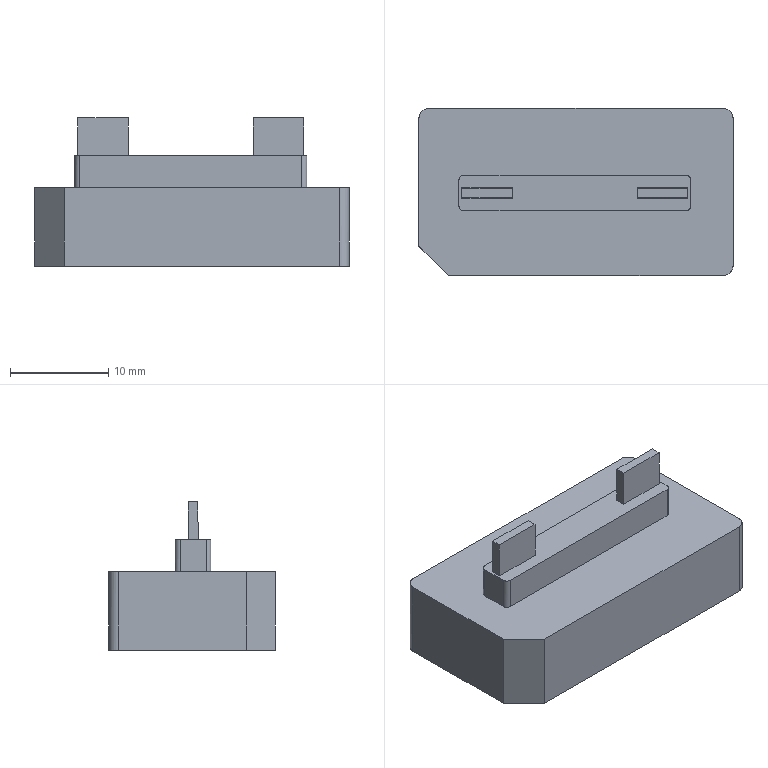NC program | PowerMill | posted by the shop | part box 32 x 17 x 15.109 mm
Lines 3099 to 3803 of 35413:
( TOOL ID   D10_1_1 )
( TOOL DIA. 10. TIP RAD 0 LENGTH 70.28 )
( Z = -4.199 )
T3 M6
T10
G91 G28 Z0
G0 G90 G54
M08
S8500 M3
X0 Y0 M8
G43 Z11.799 H3
X11.793 Y12.269
Z-2.999
G1 Z-4.199 F360
X11.412 Y7.008 F600
X8.803 Y5.703
X11.383
X11.779 Y5.688
X12.173 Y5.644
X12.562 Y5.57
X12.945 Y5.467
G2 X13.682 Y5.178 I-1.935 J-6.015
G1 X14.033 Y4.993
X14.368 Y4.782
X14.687 Y4.547
X14.988 Y4.288
X15.268 Y4.008
X15.526 Y3.707
X15.762 Y3.389
X15.973 Y3.053
X16.158 Y2.702
X16.316 Y2.339
X16.447 Y1.965
X16.55 Y1.582
X16.623 Y1.193
X16.668 Y.799
X16.683 Y.403
Y-.627
X16.668 Y-1.023
X16.623 Y-1.417
X16.55 Y-1.806
X16.447 Y-2.189
X16.316 Y-2.563
X16.158 Y-2.927
X15.973 Y-3.277
X15.762 Y-3.613
X15.526 Y-3.932
X15.268 Y-4.232
X14.988 Y-4.512
X14.687 Y-4.771
G2 X14.033 Y-5.217 I-3.905 J5.025
G1 X13.682 Y-5.402
X13.319 Y-5.561
X12.945 Y-5.692
X12.562 Y-5.794
X12.173 Y-5.868
X11.779 Y-5.912
X11.383 Y-5.927
X6.223
X5.827 Y-5.912
X5.433 Y-5.868
X5.044 Y-5.794
X4.661 Y-5.692
X4.287 Y-5.561
X3.923 Y-5.402
X3.573 Y-5.217
X3.237 Y-5.006
X2.919 Y-4.771
G2 X2.338 Y-4.232 I3.952 J4.841
G1 X2.079 Y-3.932
G2 X1.633 Y-3.277 I4.757 J3.723
G1 X1.448 Y-2.927
X1.289 Y-2.563
X1.158 Y-2.189
X1.056 Y-1.806
X.982 Y-1.417
X.938 Y-1.023
X.923 Y-.627
Y.403
X.938 Y.799
G2 X1.056 Y1.582 I6.328 J-.553
G1 X1.158 Y1.965
X1.289 Y2.339
X1.448 Y2.702
X1.633 Y3.053
X1.844 Y3.389
X2.079 Y3.707
X2.338 Y4.008
G2 X2.919 Y4.547 I4.57 J-4.343
G1 X3.237 Y4.782
X3.573 Y4.993
X3.923 Y5.178
X4.287 Y5.337
X4.661 Y5.467
X5.044 Y5.57
X5.433 Y5.644
X5.827 Y5.688
X6.223 Y5.703
X8.803
X8.869 Y5.716 Z-4.196
X8.94 Y5.768 Z-4.186
X8.978 Y5.864 Z-4.167
X8.953 Y5.964 Z-4.147
X8.889 Y6.025 Z-4.135
X8.825 Y6.046 Z-4.13
X6.619 Y6.315 Z-4.077
X6.196 Y6.335 Z-4.068
X5.767 Y6.29 Z-4.063
X5.348 Y6.18 Z-4.061
X4.952 Y6.008 Z-4.063
X4.594 Y5.783 Z-4.069
X3.226 Y4.773 Z-4.099
X3.095 Y4.677 Z-4.102 F360
X2.919 Y4.547 Z-4.105
X2.62 Y4.286 Z-4.112
X2.338 Y4.008 Z-4.119
X2.079 Y3.707 Z-4.126
X1.931 Y3.507 Z-4.131
X1.844 Y3.389 Z-4.133
X1.633 Y3.053 Z-4.14
X1.5 Y2.801 Z-4.145
X1.448 Y2.702 Z-4.147
X1.289 Y2.339 Z-4.154
X1.158 Y1.965 Z-4.161
X1.056 Y1.582 Z-4.168
X.985 Y1.192 Z-4.175
X.938 Y.799 Z-4.182
X.935 Y.73 Z-4.183
X.923 Y.403 Z-4.188
Y-.189 Z-4.199
X-1.451 Y2.115 F600
X-1.398 Y1.965
X-1.296 Y1.582
X-1.222 Y1.193
X-1.178 Y.799
X-1.163 Y.403
X-1.169 Y-.774
X-1.178 Y-1.023
X-1.222 Y-1.417
X-1.296 Y-1.806
X-1.398 Y-2.189
X-1.529 Y-2.563
X-1.688 Y-2.927
X-1.873 Y-3.277
X-2.084 Y-3.613
X-2.319 Y-3.932
X-2.578 Y-4.232
X-2.858 Y-4.512
X-3.159 Y-4.771
X-3.477 Y-5.006
X-3.813 Y-5.217
X-4.163 Y-5.402
G2 X-4.901 Y-5.692 I-2.699 J5.793
G1 X-5.284 Y-5.794
X-5.673 Y-5.868
X-6.067 Y-5.912
X-6.463 Y-5.927
X-11.623
X-12.019 Y-5.912
X-12.413 Y-5.868
G2 X-13.185 Y-5.692 I.989 J6.112
G1 X-13.559 Y-5.561
X-13.922 Y-5.402
X-14.273 Y-5.217
X-14.608 Y-5.006
X-14.927 Y-4.771
X-15.12 Y-4.606
X-15.508 Y-4.232
X-15.766 Y-3.932
G2 X-16.213 Y-3.277 I4.862 J3.795
G1 X-16.398 Y-2.927
G2 X-16.687 Y-2.189 I5.522 J2.593
G1 X-16.79 Y-1.806
X-16.863 Y-1.417
X-16.908 Y-1.023
X-16.923 Y-.627
Y.403
X-16.908 Y.799
G2 X-16.79 Y1.582 I6.194 J-.533
G1 X-16.687 Y1.965
X-16.556 Y2.339
X-16.398 Y2.703
X-16.213 Y3.053
X-16.002 Y3.389
X-15.766 Y3.707
X-15.508 Y4.008
X-15.228 Y4.288
X-14.927 Y4.547
X-14.608 Y4.782
X-14.273 Y4.993
X-13.922 Y5.178
X-13.559 Y5.337
X-13.185 Y5.467
G2 X-12.413 Y5.644 I1.802 J-6.114
G1 X-12.019 Y5.688
X-11.623 Y5.703
X-6.463
X-6.067 Y5.688
X-5.673 Y5.644
X-5.284 Y5.57
X-4.901 Y5.467
X-4.527 Y5.337
X-4.163 Y5.178
X-3.813 Y4.993
X-3.402 Y4.726
X-3.159 Y4.547
X-2.858 Y4.288
G2 X-2.319 Y3.707 I-4.255 J-4.488
G1 X-2.084 Y3.389
G2 X-1.688 Y2.702 I-5.017 J-3.354
G1 X-1.529 Y2.339
X-1.451 Y2.115
G0 Z3.999
G1 X-10.478 Y-11.178 F10000
G0 Z.849
G1 Z-.351 F360
X-10.479 Y-5.903 F600
X-10.6 Y-1.478
X-8.043 Y-1.408
G3 X-6.882 Y-.156 I-.033 J1.195
G1 X-6.892 Y.055
G3 X-8.516 Y1.112 I-1.194 J-.058
G1 X-10.932 Y.179
G3 X-10.6 Y-1.478 I.309 J-.8
G1 X-10.479 Y-5.903
G0 Z3.999
G1 X7.132 Y-11.178 F10000
G0 Z.849
G1 Z-.351 F360
X7.131 Y-5.903 F600
X7.179 Y-1.356
X9.862 Y-1.384
G3 X11.064 Y-.126 I.012 J1.192
G1 X11.055 Y.031
G3 X9.459 Y1.085 I-1.19 J-.066
G1 X6.92 Y.164
G3 X7.179 Y-1.356 I.267 J-.737
G1 X7.131 Y-5.903
G0 Z11.799
X0 Y0
Z9.799
X-21.343 Y-15.126
Z-6.11
G1 Z-7.31 F360
X-17.613 Y-11.396 F600
X-9.275 Y-7.227
X-11.423
G2 X-12.413 Y-7.138 I.053 J6.13
G1 X-12.531 Y-7.119
X-12.861 Y-7.046
X-13.186 Y-6.951
G2 X-14.271 Y-6.48 I2.079 J6.263
G1 X-14.575 Y-6.294
X-14.867 Y-6.088
G2 X-15.772 Y-5.263 I3.408 J4.644
G1 X-16.084 Y-4.871
X-16.29 Y-4.58
X-16.475 Y-4.275
X-16.64 Y-3.958
X-16.832 Y-3.509
X-16.947 Y-3.191
X-17.041 Y-2.866
G2 X-17.182 Y-2.079 I5.824 J1.45
G1 X-17.213 Y-1.754
X-17.223 Y-1.427
Y1.203
X-17.213 Y1.529
G2 X-17.041 Y2.641 I6.5 J-.431
G1 X-16.947 Y2.966
G2 X-16.607 Y3.798 I6.466 J-2.159
G1 X-16.475 Y4.051
X-16.29 Y4.356
G2 X-15.772 Y5.038 I6.341 J-4.27
G1 X-15.524 Y5.304
X-15.258 Y5.552
G2 X-14.575 Y6.07 I4.952 J-5.822
G1 X-14.271 Y6.256
X-13.954 Y6.42
G2 X-13.186 Y6.727 I3.166 J-6.809
G1 X-12.861 Y6.82
X-12.531 Y6.895
X-12.196 Y6.948
X-11.749 Y6.993
X-11.423 Y7.003
X11.183
X11.509 Y6.993
X11.858 Y6.96
G2 X12.946 Y6.727 I-.631 J-5.617
X13.714 Y6.42 I-2.451 J-7.247
X14.335 Y6.07 I-2.612 J-5.358
X15.018 Y5.552 I-4.332 J-6.423
G1 X15.284 Y5.304
X15.532 Y5.038
G2 X16.05 Y4.356 I-5.863 J-4.983
G1 X16.235 Y4.051
X16.4 Y3.734
G2 X16.707 Y2.966 I-7.095 J-3.281
G1 X16.801 Y2.641
X16.875 Y2.311
G2 X16.983 Y1.203 I-6.44 J-1.185
G1 Y-1.427
X16.973 Y-1.754
G2 X16.875 Y-2.535 I-7.272 J.511
G1 X16.8 Y-2.865
X16.707 Y-3.191
X16.543 Y-3.631
X16.4 Y-3.958
G2 X16.05 Y-4.58 I-5.365 J2.616
G1 X15.761 Y-4.98
X15.532 Y-5.263
X15.284 Y-5.528
X15.018 Y-5.776
X14.627 Y-6.088
X14.335 Y-6.294
X14.031 Y-6.48
X13.714 Y-6.644
X13.264 Y-6.836
X12.946 Y-6.951
X12.621 Y-7.045
X12.291 Y-7.119
G2 X11.509 Y-7.217 I-1.338 J7.533
G1 X11.183 Y-7.227
X-9.275
G0 Z9.799
Z10.799
X0 Y0
X14.927 Y-6.067
Z-6.08
G1 Z-7.28 F360
G3 X13.786 Y-6.191 I-.422 J-1.44 F600
G2 X11.23 Y-6.857 I-2.608 J4.768
G1 X-11.491
G2 X-16.853 Y-1.42 I.073 J5.434
G1 Y1.163
G2 X-11.488 Y6.632 I5.434 J.035
G1 X0 Y6.633
X11.233
G2 X16.613 Y1.162 I-.054 J-5.434
G1 Y-.114
Y-1.422
G2 X13.786 Y-6.191 I-5.435 J-.001
G3 X13.066 Y-7.085 I.72 J-1.316
G1 X14.837 Y-6.039
G3 X13.694 Y-6.149 I-.438 J-1.435
G2 X11.23 Y-6.777 I-2.516 J4.727
G1 X-11.488
G2 X-16.773 Y-1.42 I.07 J5.354
G1 Y1.162
G2 X-11.488 Y6.552 I5.354 J.037
G1 X0 Y6.553
X11.23
G2 X16.533 Y1.162 I-.051 J-5.354
G1 Y-.114
Y-1.42
G2 X13.694 Y-6.149 I-5.355 J-.003
G3 X12.964 Y-7.035 I.705 J-1.324
G0 Z10.799
X0 Y0
Z9.799
X21.451 Y-16.501
Z-14.01
G1 Z-15.21 F360
G3 X18.473 Y-12.484 I-1.489 J2.008 F600
G1 X18.374 Y-12.558
X18.371 Y-12.56
X18.368 Y-12.562
X17.921 Y-12.831
X17.918 Y-12.833
X17.915 Y-12.834
X17.516 Y-13.034
X17.513 Y-13.036
X17.51 Y-13.037
X17.015 Y-13.235
X17.012 Y-13.236
X17.009 Y-13.237
X16.562 Y-13.375
X16.559 Y-13.376
X16.556 Y-13.377
X16.053 Y-13.488
X16.05
X16.047 Y-13.489
X15.656 Y-13.544
X15.653
X15.65
X15.203 Y-13.576
X15.201
X15.198
X14.751 Y-13.58
X-12.963
X-12.964
X-12.966
X-13.413 Y-13.563
X-13.416
X-13.42
X-13.867 Y-13.505
X-13.87
X-13.874 Y-13.504
X-14.321 Y-13.405
X-14.324 Y-13.404
X-14.328 Y-13.403
X-14.775 Y-13.26
X-14.779 Y-13.258
X-14.782 Y-13.257
X-15.229 Y-13.065
X-15.233 Y-13.063
X-15.236 Y-13.061
X-15.683 Y-12.813
X-15.686 Y-12.812
X-15.69 Y-12.81
X-16.024 Y-12.582
X-16.026 Y-12.58
X-16.028 Y-12.579
X-16.14 Y-12.493
X-16.142 Y-12.492
X-16.144 Y-12.49
X-16.555 Y-12.129
X-16.557 Y-12.127
X-16.559 Y-12.125
X-19.241 Y-9.443
X-19.686 Y-8.996
X-19.688 Y-8.994
X-19.69 Y-8.991
X-20.067 Y-8.544
X-20.069 Y-8.542
X-20.07 Y-8.539
X-20.179 Y-8.388
X-20.181 Y-8.386
X-20.182 Y-8.384
X-20.371 Y-8.089
X-20.373 Y-8.086
X-20.374 Y-8.083
X-20.609 Y-7.636
X-20.611 Y-7.632
X-20.612 Y-7.629
X-20.793 Y-7.182
X-20.795 Y-7.178
X-20.796 Y-7.175
X-20.929 Y-6.728
X-20.93 Y-6.724
X-20.931 Y-6.72
X-21.021 Y-6.274
Y-6.27
X-21.022 Y-6.266
X-21.07 Y-5.819
Y-5.816
Y-5.813
X-21.08 Y-5.366
Y-5.365
Y-5.364
X-21.079 Y7.599
Y7.601
Y7.603
X-21.053 Y8.05
Y8.053
Y8.056
X-20.996 Y8.503
Y8.506
X-20.995 Y8.509
X-20.902 Y8.956
X-20.901 Y8.959
X-20.9 Y8.962
X-20.772 Y9.409
X-20.771 Y9.412
X-20.77 Y9.414
X-20.636 Y9.78
X-20.635 Y9.783
X-20.634 Y9.786
X-20.389 Y10.314
X-20.387 Y10.318
X-20.386 Y10.321
X-20.127 Y10.768
X-20.125 Y10.771
X-20.123 Y10.774
X-19.807 Y11.221
X-19.805 Y11.224
X-19.803 Y11.227
X-19.42 Y11.674
X-19.419 Y11.676
X-19.417 Y11.677
X-19.278 Y11.821
X-19.276 Y11.823
X-19.274 Y11.825
X-18.827 Y12.222
X-18.824 Y12.224
X-18.821 Y12.226
X-18.374 Y12.558
X-18.371 Y12.56
X-18.368 Y12.562
X-17.921 Y12.831
X-17.918 Y12.833
X-17.915 Y12.834
X-17.516 Y13.034
X-17.513 Y13.036
X-17.51 Y13.037
X-17.015 Y13.235
X-17.012 Y13.236
X-17.009 Y13.237
X-16.562 Y13.375
X-16.559 Y13.376
X-16.556 Y13.377
X-16.109 Y13.478
X-16.106
X-16.103 Y13.479
X-15.656 Y13.544
X-15.653
X-15.65
X-15.203 Y13.576
X-15.201
X-15.198
X-14.751 Y13.58
X0
X14.751
X15.198 Y13.576
X15.201
X15.203
X15.65 Y13.544
X15.653
X15.656
X16.047 Y13.489
X16.05 Y13.488
X16.053
X16.556 Y13.377
X16.559 Y13.376
X16.562 Y13.375
X17.009 Y13.237
X17.012
X17.015 Y13.235
X17.462 Y13.059
X17.465 Y13.058
X17.468 Y13.056
X17.915 Y12.834
X17.918 Y12.833
X17.92 Y12.831
X18.334 Y12.584
X18.337 Y12.582
X18.34 Y12.58
X18.821 Y12.227
X18.824 Y12.224
X18.827 Y12.222
X19.274 Y11.825
X19.276 Y11.823
X19.278 Y11.821
X19.417 Y11.677
X19.419 Y11.676
X19.42 Y11.674
X19.803 Y11.227
X19.805 Y11.224
X19.807 Y11.221
X20.123 Y10.774
X20.125 Y10.771
X20.127 Y10.768
X20.386 Y10.321
X20.387 Y10.318
X20.389 Y10.315
X20.6 Y9.868
X20.601 Y9.865
X20.602 Y9.862
X20.77 Y9.415
X20.771 Y9.412
X20.772 Y9.409
X20.9 Y8.962
X20.901 Y8.959
X20.902 Y8.956
X20.995 Y8.509
X20.996 Y8.506
Y8.503
X21.053 Y8.056
Y8.053
Y8.05
X21.079 Y7.603
Y7.601
Y7.599
Y-7.599
Y-7.601
Y-7.603
X21.053 Y-8.05
Y-8.053
Y-8.056
X20.996 Y-8.503
Y-8.506
X20.995 Y-8.509
X20.902 Y-8.956
X20.901 Y-8.959
X20.9 Y-8.962
X20.772 Y-9.409
X20.771 Y-9.412
X20.77 Y-9.414
X20.636 Y-9.78
X20.635 Y-9.783
X20.634 Y-9.786
X20.389 Y-10.314
X20.387 Y-10.318
X20.386 Y-10.321
X20.127 Y-10.768
X20.125 Y-10.771
X20.123 Y-10.774
X19.807 Y-11.221
X19.805 Y-11.224
X19.803 Y-11.227
X19.42 Y-11.674
X19.419 Y-11.676
X19.417 Y-11.677
X19.278 Y-11.821
X19.276 Y-11.823
X19.274 Y-11.825
X18.827 Y-12.222
X18.824 Y-12.224
X18.821 Y-12.226
X18.473 Y-12.484
G3 X21.451 Y-16.501 I1.489 J-2.008
G1 X21.399 Y-16.439
G3 X18.422 Y-12.423 I-1.489 J2.008
G1 X18.326 Y-12.494
X17.879 Y-12.763
X17.481 Y-12.963
X16.985 Y-13.161
X16.538 Y-13.298
X16.036 Y-13.41
X15.644 Y-13.464
X15.198 Y-13.496
X14.751 Y-13.5
X-12.963
X-13.41 Y-13.483
X-13.857 Y-13.426
X-14.304 Y-13.327
X-14.751 Y-13.184
X-15.198 Y-12.991
X-15.644 Y-12.743
X-15.979 Y-12.516
X-16.091 Y-12.43
X-16.502 Y-12.069
X-19.184 Y-9.387
X-19.629 Y-8.94
X-20.005 Y-8.493
X-20.114 Y-8.341
X-20.303 Y-8.046
X-20.538 Y-7.599
X-20.719 Y-7.152
X-20.853 Y-6.705
X-20.942 Y-6.258
X-20.99 Y-5.811
X-21. Y-5.364
X-20.999 Y7.599
X-20.973 Y8.046
X-20.917 Y8.493
X-20.823 Y8.94
X-20.695 Y9.387
X-20.561 Y9.752
X-20.316 Y10.281
X-20.058 Y10.728
X-19.742 Y11.175
X-19.36 Y11.622
X-19.22 Y11.765
X-18.773 Y12.162
X-18.326 Y12.494
X-17.879 Y12.763
X-17.481 Y12.963
X-16.985 Y13.161
X-16.538 Y13.298
X-16.091 Y13.4
X-15.644 Y13.464
X-15.198 Y13.496
X-14.751 Y13.5
X0
X14.751
X15.198 Y13.496
X15.644 Y13.464
X16.036 Y13.41
X16.538 Y13.298
X16.985 Y13.161
X17.432 Y12.984
X17.879 Y12.763
X18.293 Y12.516
X18.773 Y12.162
X19.22 Y11.765
X19.36 Y11.622
X19.742 Y11.175
X20.058 Y10.728
X20.316 Y10.281
X20.528 Y9.834
X20.695 Y9.387
X20.823 Y8.94
X20.917 Y8.493
X20.973 Y8.046
X20.999 Y7.599
Y-7.599
X20.973 Y-8.046
X20.917 Y-8.493
X20.823 Y-8.94
X20.695 Y-9.387
X20.561 Y-9.752
X20.316 Y-10.281
X20.058 Y-10.728
X19.742 Y-11.175
X19.36 Y-11.622
X19.22 Y-11.765
X18.773 Y-12.162
X18.422 Y-12.423
G3 X21.399 Y-16.439 I1.489 J-2.008
G0 Z9.799
Z10.799
X0 Y0
M9
M5
M01